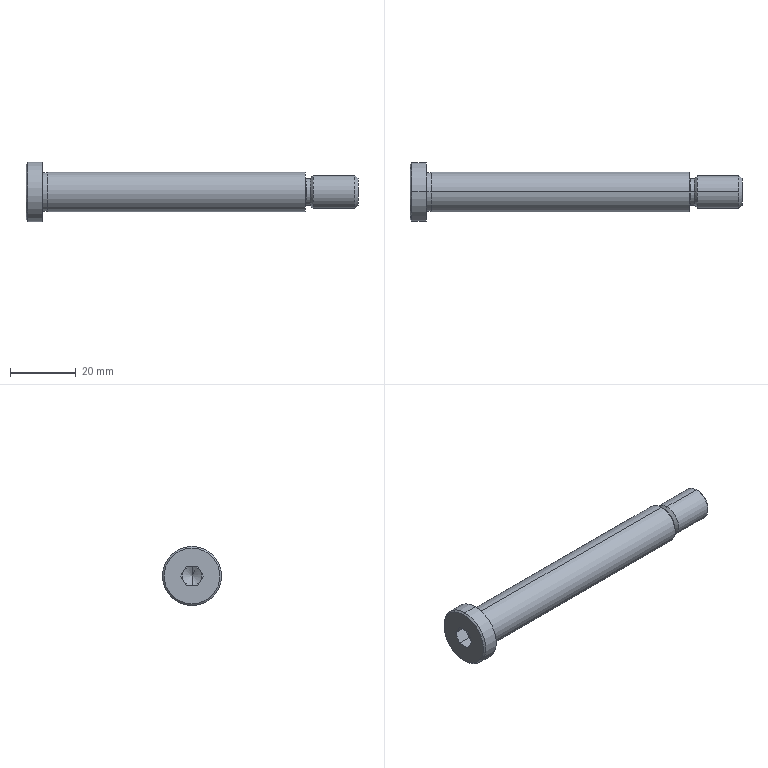Part | STEP file | 001-009-MIJ04-D12-L80 | 1 solid | 39 faces | box 101 x 18 x 18 mm | volume 11360 mm3 | plane 17 | cylinder 10 | cone 8 | torus 4 | commonest cylinder face diameters 8.2 x2 10 x2 11.8 x2 12 x2 18 x2